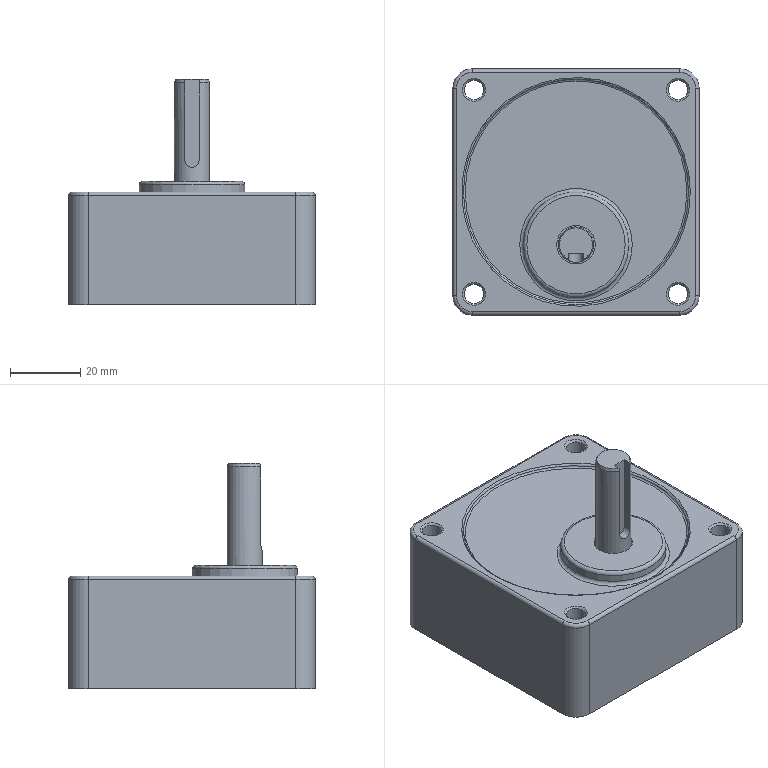Part | STEP file | S7KA3-18 | 1 solid | 46 faces | box 70 x 70 x 64 mm | volume 137824 mm3 | cylinder 18 | plane 15 | torus 8 | cone 5 | commonest cylinder face diameters 11 x5 2 x4 5.5 x4 4 x1 7 x1 10 x1
STEP:
#1=CARTESIAN_POINT('',(31.5,35.,5.));
#2=VERTEX_POINT('',#1);
#3=CARTESIAN_POINT('',(35.,35.,5.));
#4=DIRECTION('',(0.,0.,1.));
#5=DIRECTION('',(1.,0.,0.));
#6=AXIS2_PLACEMENT_3D('',#3,#4,#5);
#7=CIRCLE('',#6,3.5);
#8=EDGE_CURVE('',#2,#2,#7,.T.);
#9=ORIENTED_EDGE('',*,*,#8,.F.);
#10=CARTESIAN_POINT('',(31.5,35.,19.));
#11=VERTEX_POINT('',#10);
#12=CARTESIAN_POINT('',(31.5,35.,5.));
#13=DIRECTION('',(0.,0.,1.));
#14=VECTOR('',#13,3.5);
#15=LINE('',#12,#14);
#16=EDGE_CURVE('',#2,#11,#15,.T.);
#17=ORIENTED_EDGE('',*,*,#16,.T.);
#18=CARTESIAN_POINT('',(35.,35.,19.));
#19=DIRECTION('',(0.,0.,-1.));
#20=DIRECTION('',(1.,0.,0.));
#21=AXIS2_PLACEMENT_3D('',#18,#19,#20);
#22=CIRCLE('',#21,3.5);
#23=EDGE_CURVE('',#11,#11,#22,.T.);
#24=ORIENTED_EDGE('',*,*,#23,.F.);
#25=ORIENTED_EDGE('',*,*,#16,.F.);
#26=EDGE_LOOP('',(#9,#17,#24,#25));
#27=FACE_OUTER_BOUND('',#26,.T.);
#28=CARTESIAN_POINT('',(35.,35.,5.));
#29=DIRECTION('',(0.,0.,1.));
#30=DIRECTION('',(1.,0.,0.));
#31=AXIS2_PLACEMENT_3D('',#28,#29,#30);
#32=CYLINDRICAL_SURFACE('',#31,3.5);
#33=ADVANCED_FACE('',(#27),#32,.F.);
#34=ORIENTED_EDGE('',*,*,#23,.T.);
#35=EDGE_LOOP('',(#34));
#36=FACE_OUTER_BOUND('',#35,.T.);
#37=CARTESIAN_POINT('',(35.,35.,19.));
#38=DIRECTION('',(0.,0.,1.));
#39=DIRECTION('',(1.,0.,0.));
#40=AXIS2_PLACEMENT_3D('',#37,#38,#39);
#41=PLANE('',#40);
#42=ADVANCED_FACE('',(#36),#41,.F.);
#43=CARTESIAN_POINT('',(3.,35.,0.));
#44=VERTEX_POINT('',#43);
#45=CARTESIAN_POINT('',(35.,35.,0.));
#46=DIRECTION('',(0.,0.,1.));
#47=DIRECTION('',(1.,0.,0.));
#48=AXIS2_PLACEMENT_3D('',#45,#46,#47);
#49=CIRCLE('',#48,32.);
#50=EDGE_CURVE('',#44,#44,#49,.T.);
#51=ORIENTED_EDGE('',*,*,#50,.F.);
#52=CARTESIAN_POINT('',(3.,35.,5.));
#53=VERTEX_POINT('',#52);
#54=CARTESIAN_POINT('',(3.,35.,0.));
#55=DIRECTION('',(0.,0.,1.));
#56=VECTOR('',#55,32.);
#57=LINE('',#54,#56);
#58=EDGE_CURVE('',#44,#53,#57,.T.);
#59=ORIENTED_EDGE('',*,*,#58,.T.);
#60=CARTESIAN_POINT('',(35.,35.,5.));
#61=DIRECTION('',(0.,0.,-1.));
#62=DIRECTION('',(1.,0.,0.));
#63=AXIS2_PLACEMENT_3D('',#60,#61,#62);
#64=CIRCLE('',#63,32.);
#65=EDGE_CURVE('',#53,#53,#64,.T.);
#66=ORIENTED_EDGE('',*,*,#65,.F.);
#67=ORIENTED_EDGE('',*,*,#58,.F.);
#68=EDGE_LOOP('',(#51,#59,#66,#67));
#69=FACE_OUTER_BOUND('',#68,.T.);
#70=CARTESIAN_POINT('',(35.,35.,0.));
#71=DIRECTION('',(0.,0.,1.));
#72=DIRECTION('',(1.,0.,0.));
#73=AXIS2_PLACEMENT_3D('',#70,#71,#72);
#74=CYLINDRICAL_SURFACE('',#73,32.);
#75=ADVANCED_FACE('',(#69),#74,.F.);
#76=ORIENTED_EDGE('',*,*,#65,.T.);
#77=EDGE_LOOP('',(#76));
#78=FACE_OUTER_BOUND('',#77,.T.);
#79=ORIENTED_EDGE('',*,*,#8,.T.);
#80=EDGE_LOOP('',(#79));
#81=FACE_BOUND('',#80,.T.);
#82=CARTESIAN_POINT('',(35.,35.,5.));
#83=DIRECTION('',(0.,0.,1.));
#84=DIRECTION('',(1.,0.,0.));
#85=AXIS2_PLACEMENT_3D('',#82,#83,#84);
#86=PLANE('',#85);
#87=ADVANCED_FACE('',(#78,#81),#86,.F.);
#88=CARTESIAN_POINT('',(66.741,6.009,31.5));
#89=VERTEX_POINT('',#88);
#90=CARTESIAN_POINT('',(63.991,6.009,31.5));
#91=DIRECTION('',(0.,0.,-1.));
#92=DIRECTION('',(-1.,0.,0.));
#93=AXIS2_PLACEMENT_3D('',#90,#91,#92);
#94=CIRCLE('',#93,2.75);
#95=EDGE_CURVE('',#89,#89,#94,.T.);
#96=ORIENTED_EDGE('',*,*,#95,.T.);
#97=CARTESIAN_POINT('',(67.241,6.009,32.));
#98=VERTEX_POINT('',#97);
#99=CARTESIAN_POINT('',(66.991,6.009,31.75));
#100=DIRECTION('',(0.7071,0.,0.7071));
#101=VECTOR('',#100,3.);
#102=LINE('',#99,#101);
#103=EDGE_CURVE('',#89,#98,#102,.T.);
#104=ORIENTED_EDGE('',*,*,#103,.T.);
#105=CARTESIAN_POINT('',(63.991,6.009,32.));
#106=DIRECTION('',(0.,0.,1.));
#107=DIRECTION('',(-1.,0.,0.));
#108=AXIS2_PLACEMENT_3D('',#105,#106,#107);
#109=CIRCLE('',#108,3.25);
#110=EDGE_CURVE('',#98,#98,#109,.T.);
#111=ORIENTED_EDGE('',*,*,#110,.T.);
#112=ORIENTED_EDGE('',*,*,#103,.F.);
#113=EDGE_LOOP('',(#96,#104,#111,#112));
#114=FACE_OUTER_BOUND('',#113,.T.);
#115=CARTESIAN_POINT('',(63.991,6.009,31.75));
#116=DIRECTION('',(0.,0.,1.));
#117=DIRECTION('',(-1.,0.,0.));
#118=AXIS2_PLACEMENT_3D('',#115,#116,#117);
#119=CONICAL_SURFACE('',#118,3.,0.7854);
#120=ADVANCED_FACE('',(#114),#119,.F.);
#121=CARTESIAN_POINT('',(64.5,1.,32.));
#122=VERTEX_POINT('',#121);
#123=CARTESIAN_POINT('',(5.5,1.,32.));
#124=VERTEX_POINT('',#123);
#125=CARTESIAN_POINT('',(64.5,1.,32.));
#126=DIRECTION('',(-1.,0.,0.));
#127=VECTOR('',#126,59.);
#128=LINE('',#125,#127);
#129=EDGE_CURVE('',#122,#124,#128,.T.);
#130=ORIENTED_EDGE('',*,*,#129,.F.);
#131=CARTESIAN_POINT('',(69.,5.5,32.));
#132=VERTEX_POINT('',#131);
#133=CARTESIAN_POINT('',(64.5,5.5,32.));
#134=DIRECTION('',(0.,0.,-1.));
#135=DIRECTION('',(0.7071,-0.7071,0.));
#136=AXIS2_PLACEMENT_3D('',#133,#134,#135);
#137=CIRCLE('',#136,4.5);
#138=EDGE_CURVE('',#132,#122,#137,.T.);
#139=ORIENTED_EDGE('',*,*,#138,.F.);
#140=CARTESIAN_POINT('',(69.,64.5,32.));
#141=VERTEX_POINT('',#140);
#142=CARTESIAN_POINT('',(69.,64.5,32.));
#143=DIRECTION('',(0.,-1.,0.));
#144=VECTOR('',#143,59.);
#145=LINE('',#142,#144);
#146=EDGE_CURVE('',#141,#132,#145,.T.);
#147=ORIENTED_EDGE('',*,*,#146,.F.);
#148=CARTESIAN_POINT('',(64.5,69.,32.));
#149=VERTEX_POINT('',#148);
#150=CARTESIAN_POINT('',(64.5,64.5,32.));
#151=DIRECTION('',(0.,0.,-1.));
#152=DIRECTION('',(0.7071,0.7071,0.));
#153=AXIS2_PLACEMENT_3D('',#150,#151,#152);
#154=CIRCLE('',#153,4.5);
#155=EDGE_CURVE('',#149,#141,#154,.T.);
#156=ORIENTED_EDGE('',*,*,#155,.F.);
#157=CARTESIAN_POINT('',(5.5,69.,32.));
#158=VERTEX_POINT('',#157);
#159=CARTESIAN_POINT('',(5.5,69.,32.));
#160=DIRECTION('',(1.,0.,0.));
#161=VECTOR('',#160,59.);
#162=LINE('',#159,#161);
#163=EDGE_CURVE('',#158,#149,#162,.T.);
#164=ORIENTED_EDGE('',*,*,#163,.F.);
#165=CARTESIAN_POINT('',(1.,64.5,32.));
#166=VERTEX_POINT('',#165);
#167=CARTESIAN_POINT('',(5.5,64.5,32.));
#168=DIRECTION('',(0.,0.,-1.));
#169=DIRECTION('',(-0.7071,0.7071,0.));
#170=AXIS2_PLACEMENT_3D('',#167,#168,#169);
#171=CIRCLE('',#170,4.5);
#172=EDGE_CURVE('',#166,#158,#171,.T.);
#173=ORIENTED_EDGE('',*,*,#172,.F.);
#174=CARTESIAN_POINT('',(1.,5.5,32.));
#175=VERTEX_POINT('',#174);
#176=CARTESIAN_POINT('',(1.,5.5,32.));
#177=DIRECTION('',(0.,1.,0.));
#178=VECTOR('',#177,59.);
#179=LINE('',#176,#178);
#180=EDGE_CURVE('',#175,#166,#179,.T.);
#181=ORIENTED_EDGE('',*,*,#180,.F.);
#182=CARTESIAN_POINT('',(5.5,5.5,32.));
#183=DIRECTION('',(0.,0.,-1.));
#184=DIRECTION('',(-0.7071,-0.7071,0.));
#185=AXIS2_PLACEMENT_3D('',#182,#183,#184);
#186=CIRCLE('',#185,4.5);
#187=EDGE_CURVE('',#124,#175,#186,.T.);
#188=ORIENTED_EDGE('',*,*,#187,.F.);
#189=EDGE_LOOP('',(#130,#139,#147,#156,#164,#173,#181,#188));
#190=FACE_OUTER_BOUND('',#189,.T.);
#191=CARTESIAN_POINT('',(9.259,6.009,32.));
#192=VERTEX_POINT('',#191);
#193=CARTESIAN_POINT('',(6.009,6.009,32.));
#194=DIRECTION('',(0.,0.,1.));
#195=DIRECTION('',(-1.,0.,0.));
#196=AXIS2_PLACEMENT_3D('',#193,#194,#195);
#197=CIRCLE('',#196,3.25);
#198=EDGE_CURVE('',#192,#192,#197,.T.);
#199=ORIENTED_EDGE('',*,*,#198,.F.);
#200=EDGE_LOOP('',(#199));
#201=FACE_BOUND('',#200,.T.);
#202=CARTESIAN_POINT('',(67.241,63.991,32.));
#203=VERTEX_POINT('',#202);
#204=CARTESIAN_POINT('',(63.991,63.991,32.));
#205=DIRECTION('',(0.,0.,1.));
#206=DIRECTION('',(-1.,0.,0.));
#207=AXIS2_PLACEMENT_3D('',#204,#205,#206);
#208=CIRCLE('',#207,3.25);
#209=EDGE_CURVE('',#203,#203,#208,.T.);
#210=ORIENTED_EDGE('',*,*,#209,.F.);
#211=EDGE_LOOP('',(#210));
#212=FACE_BOUND('',#211,.T.);
#213=CARTESIAN_POINT('',(67.5,35.,32.));
#214=VERTEX_POINT('',#213);
#215=CARTESIAN_POINT('',(35.,35.,32.));
#216=DIRECTION('',(0.,0.,1.));
#217=DIRECTION('',(-1.,0.,0.));
#218=AXIS2_PLACEMENT_3D('',#215,#216,#217);
#219=CIRCLE('',#218,32.5);
#220=EDGE_CURVE('',#214,#214,#219,.T.);
#221=ORIENTED_EDGE('',*,*,#220,.F.);
#222=EDGE_LOOP('',(#221));
#223=FACE_BOUND('',#222,.T.);
#224=CARTESIAN_POINT('',(9.259,63.991,32.));
#225=VERTEX_POINT('',#224);
#226=CARTESIAN_POINT('',(6.009,63.991,32.));
#227=DIRECTION('',(0.,0.,1.));
#228=DIRECTION('',(-1.,0.,0.));
#229=AXIS2_PLACEMENT_3D('',#226,#227,#228);
#230=CIRCLE('',#229,3.25);
#231=EDGE_CURVE('',#225,#225,#230,.T.);
#232=ORIENTED_EDGE('',*,*,#231,.F.);
#233=EDGE_LOOP('',(#232));
#234=FACE_BOUND('',#233,.T.);
#235=ORIENTED_EDGE('',*,*,#110,.F.);
#236=EDGE_LOOP('',(#235));
#237=FACE_BOUND('',#236,.T.);
#238=CARTESIAN_POINT('',(35.,35.,32.));
#239=DIRECTION('',(0.,0.,1.));
#240=DIRECTION('',(1.,0.,0.));
#241=AXIS2_PLACEMENT_3D('',#238,#239,#240);
#242=PLANE('',#241);
#243=ADVANCED_FACE('',(#190,#201,#212,#223,#234,#237),#242,.T.);
#244=ORIENTED_EDGE('',*,*,#95,.F.);
#245=CARTESIAN_POINT('',(66.741,6.009,0.));
#246=VERTEX_POINT('',#245);
#247=CARTESIAN_POINT('',(66.741,6.009,32.));
#248=DIRECTION('',(0.,0.,-1.));
#249=VECTOR('',#248,2.75);
#250=LINE('',#247,#249);
#251=EDGE_CURVE('',#89,#246,#250,.T.);
#252=ORIENTED_EDGE('',*,*,#251,.T.);
#253=CARTESIAN_POINT('',(63.991,6.009,0.));
#254=DIRECTION('',(0.,0.,1.));
#255=DIRECTION('',(-1.,0.,0.));
#256=AXIS2_PLACEMENT_3D('',#253,#254,#255);
#257=CIRCLE('',#256,2.75);
#258=EDGE_CURVE('',#246,#246,#257,.T.);
#259=ORIENTED_EDGE('',*,*,#258,.F.);
#260=ORIENTED_EDGE('',*,*,#251,.F.);
#261=EDGE_LOOP('',(#244,#252,#259,#260));
#262=FACE_OUTER_BOUND('',#261,.T.);
#263=CARTESIAN_POINT('',(63.991,6.009,32.));
#264=DIRECTION('',(0.,0.,-1.));
#265=DIRECTION('',(-1.,0.,0.));
#266=AXIS2_PLACEMENT_3D('',#263,#264,#265);
#267=CYLINDRICAL_SURFACE('',#266,2.75);
#268=ADVANCED_FACE('',(#262),#267,.F.);
#269=CARTESIAN_POINT('',(8.759,6.009,31.5));
#270=VERTEX_POINT('',#269);
#271=CARTESIAN_POINT('',(6.009,6.009,31.5));
#272=DIRECTION('',(0.,0.,-1.));
#273=DIRECTION('',(-1.,0.,0.));
#274=AXIS2_PLACEMENT_3D('',#271,#272,#273);
#275=CIRCLE('',#274,2.75);
#276=EDGE_CURVE('',#270,#270,#275,.T.);
#277=ORIENTED_EDGE('',*,*,#276,.T.);
#278=CARTESIAN_POINT('',(9.009,6.009,31.75));
#279=DIRECTION('',(0.7071,0.,0.7071));
#280=VECTOR('',#279,3.);
#281=LINE('',#278,#280);
#282=EDGE_CURVE('',#270,#192,#281,.T.);
#283=ORIENTED_EDGE('',*,*,#282,.T.);
#284=ORIENTED_EDGE('',*,*,#198,.T.);
#285=ORIENTED_EDGE('',*,*,#282,.F.);
#286=EDGE_LOOP('',(#277,#283,#284,#285));
#287=FACE_OUTER_BOUND('',#286,.T.);
#288=CARTESIAN_POINT('',(6.009,6.009,31.75));
#289=DIRECTION('',(0.,0.,1.));
#290=DIRECTION('',(-1.,0.,0.));
#291=AXIS2_PLACEMENT_3D('',#288,#289,#290);
#292=CONICAL_SURFACE('',#291,3.,0.7854);
#293=ADVANCED_FACE('',(#287),#292,.F.);
#294=ORIENTED_EDGE('',*,*,#276,.F.);
#295=CARTESIAN_POINT('',(8.759,6.009,0.));
#296=VERTEX_POINT('',#295);
#297=CARTESIAN_POINT('',(8.759,6.009,32.));
#298=DIRECTION('',(0.,0.,-1.));
#299=VECTOR('',#298,2.75);
#300=LINE('',#297,#299);
#301=EDGE_CURVE('',#270,#296,#300,.T.);
#302=ORIENTED_EDGE('',*,*,#301,.T.);
#303=CARTESIAN_POINT('',(6.009,6.009,0.));
#304=DIRECTION('',(0.,0.,1.));
#305=DIRECTION('',(-1.,0.,0.));
#306=AXIS2_PLACEMENT_3D('',#303,#304,#305);
#307=CIRCLE('',#306,2.75);
#308=EDGE_CURVE('',#296,#296,#307,.T.);
#309=ORIENTED_EDGE('',*,*,#308,.F.);
#310=ORIENTED_EDGE('',*,*,#301,.F.);
#311=EDGE_LOOP('',(#294,#302,#309,#310));
#312=FACE_OUTER_BOUND('',#311,.T.);
#313=CARTESIAN_POINT('',(6.009,6.009,32.));
#314=DIRECTION('',(0.,0.,-1.));
#315=DIRECTION('',(-1.,0.,0.));
#316=AXIS2_PLACEMENT_3D('',#313,#314,#315);
#317=CYLINDRICAL_SURFACE('',#316,2.75);
#318=ADVANCED_FACE('',(#312),#317,.F.);
#319=CARTESIAN_POINT('',(8.759,63.991,31.5));
#320=VERTEX_POINT('',#319);
#321=CARTESIAN_POINT('',(6.009,63.991,31.5));
#322=DIRECTION('',(0.,0.,-1.));
#323=DIRECTION('',(-1.,0.,0.));
#324=AXIS2_PLACEMENT_3D('',#321,#322,#323);
#325=CIRCLE('',#324,2.75);
#326=EDGE_CURVE('',#320,#320,#325,.T.);
#327=ORIENTED_EDGE('',*,*,#326,.T.);
#328=CARTESIAN_POINT('',(9.009,63.991,31.75));
#329=DIRECTION('',(0.7071,0.,0.7071));
#330=VECTOR('',#329,3.);
#331=LINE('',#328,#330);
#332=EDGE_CURVE('',#320,#225,#331,.T.);
#333=ORIENTED_EDGE('',*,*,#332,.T.);
#334=ORIENTED_EDGE('',*,*,#231,.T.);
#335=ORIENTED_EDGE('',*,*,#332,.F.);
#336=EDGE_LOOP('',(#327,#333,#334,#335));
#337=FACE_OUTER_BOUND('',#336,.T.);
#338=CARTESIAN_POINT('',(6.009,63.991,31.75));
#339=DIRECTION('',(0.,0.,1.));
#340=DIRECTION('',(-1.,0.,0.));
#341=AXIS2_PLACEMENT_3D('',#338,#339,#340);
#342=CONICAL_SURFACE('',#341,3.,0.7854);
#343=ADVANCED_FACE('',(#337),#342,.F.);
#344=ORIENTED_EDGE('',*,*,#326,.F.);
#345=CARTESIAN_POINT('',(8.759,63.991,0.));
#346=VERTEX_POINT('',#345);
#347=CARTESIAN_POINT('',(8.759,63.991,32.));
#348=DIRECTION('',(0.,0.,-1.));
#349=VECTOR('',#348,2.75);
#350=LINE('',#347,#349);
#351=EDGE_CURVE('',#320,#346,#350,.T.);
#352=ORIENTED_EDGE('',*,*,#351,.T.);
#353=CARTESIAN_POINT('',(6.009,63.991,0.));
#354=DIRECTION('',(0.,0.,1.));
#355=DIRECTION('',(-1.,0.,0.));
#356=AXIS2_PLACEMENT_3D('',#353,#354,#355);
#357=CIRCLE('',#356,2.75);
#358=EDGE_CURVE('',#346,#346,#357,.T.);
#359=ORIENTED_EDGE('',*,*,#358,.F.);
#360=ORIENTED_EDGE('',*,*,#351,.F.);
#361=EDGE_LOOP('',(#344,#352,#359,#360));
#362=FACE_OUTER_BOUND('',#361,.T.);
#363=CARTESIAN_POINT('',(6.009,63.991,32.));
#364=DIRECTION('',(0.,0.,-1.));
#365=DIRECTION('',(-1.,0.,0.));
#366=AXIS2_PLACEMENT_3D('',#363,#364,#365);
#367=CYLINDRICAL_SURFACE('',#366,2.75);
#368=ADVANCED_FACE('',(#362),#367,.F.);
#369=CARTESIAN_POINT('',(66.741,63.991,31.5));
#370=VERTEX_POINT('',#369);
#371=CARTESIAN_POINT('',(63.991,63.991,31.5));
#372=DIRECTION('',(0.,0.,-1.));
#373=DIRECTION('',(-1.,0.,0.));
#374=AXIS2_PLACEMENT_3D('',#371,#372,#373);
#375=CIRCLE('',#374,2.75);
#376=EDGE_CURVE('',#370,#370,#375,.T.);
#377=ORIENTED_EDGE('',*,*,#376,.T.);
#378=CARTESIAN_POINT('',(66.991,63.991,31.75));
#379=DIRECTION('',(0.7071,0.,0.7071));
#380=VECTOR('',#379,3.);
#381=LINE('',#378,#380);
#382=EDGE_CURVE('',#370,#203,#381,.T.);
#383=ORIENTED_EDGE('',*,*,#382,.T.);
#384=ORIENTED_EDGE('',*,*,#209,.T.);
#385=ORIENTED_EDGE('',*,*,#382,.F.);
#386=EDGE_LOOP('',(#377,#383,#384,#385));
#387=FACE_OUTER_BOUND('',#386,.T.);
#388=CARTESIAN_POINT('',(63.991,63.991,31.75));
#389=DIRECTION('',(0.,0.,1.));
#390=DIRECTION('',(-1.,0.,0.));
#391=AXIS2_PLACEMENT_3D('',#388,#389,#390);
#392=CONICAL_SURFACE('',#391,3.,0.7854);
#393=ADVANCED_FACE('',(#387),#392,.F.);
#394=ORIENTED_EDGE('',*,*,#376,.F.);
#395=CARTESIAN_POINT('',(66.741,63.991,0.));
#396=VERTEX_POINT('',#395);
#397=CARTESIAN_POINT('',(66.741,63.991,32.));
#398=DIRECTION('',(0.,0.,-1.));
#399=VECTOR('',#398,2.75);
#400=LINE('',#397,#399);
#401=EDGE_CURVE('',#370,#396,#400,.T.);
#402=ORIENTED_EDGE('',*,*,#401,.T.);
#403=CARTESIAN_POINT('',(63.991,63.991,0.));
#404=DIRECTION('',(0.,0.,1.));
#405=DIRECTION('',(-1.,0.,0.));
#406=AXIS2_PLACEMENT_3D('',#403,#404,#405);
#407=CIRCLE('',#406,2.75);
#408=EDGE_CURVE('',#396,#396,#407,.T.);
#409=ORIENTED_EDGE('',*,*,#408,.F.);
#410=ORIENTED_EDGE('',*,*,#401,.F.);
#411=EDGE_LOOP('',(#394,#402,#409,#410));
#412=FACE_OUTER_BOUND('',#411,.T.);
#413=CARTESIAN_POINT('',(63.991,63.991,32.));
#414=DIRECTION('',(0.,0.,-1.));
#415=DIRECTION('',(-1.,0.,0.));
#416=AXIS2_PLACEMENT_3D('',#413,#414,#415);
#417=CYLINDRICAL_SURFACE('',#416,2.75);
#418=ADVANCED_FACE('',(#412),#417,.F.);
#419=CARTESIAN_POINT('',(33.,15.417,41.));
#420=VERTEX_POINT('',#419);
#421=CARTESIAN_POINT('',(33.,15.417,63.));
#422=VERTEX_POINT('',#421);
#423=CARTESIAN_POINT('',(33.,15.417,41.));
#424=DIRECTION('',(0.,0.,1.));
#425=VECTOR('',#424,22.);
#426=LINE('',#423,#425);
#427=EDGE_CURVE('',#420,#422,#426,.T.);
#428=ORIENTED_EDGE('',*,*,#427,.F.);
#429=CARTESIAN_POINT('',(33.,17.5,41.));
#430=VERTEX_POINT('',#429);
#431=CARTESIAN_POINT('',(33.,15.417,41.));
#432=DIRECTION('',(0.,1.,0.));
#433=VECTOR('',#432,2.083);
#434=LINE('',#431,#433);
#435=EDGE_CURVE('',#420,#430,#434,.T.);
#436=ORIENTED_EDGE('',*,*,#435,.T.);
#437=CARTESIAN_POINT('',(33.,17.5,64.));
#438=VERTEX_POINT('',#437);
#439=CARTESIAN_POINT('',(33.,17.5,64.));
#440=DIRECTION('',(0.,0.,-1.));
#441=VECTOR('',#440,23.);
#442=LINE('',#439,#441);
#443=EDGE_CURVE('',#438,#430,#442,.T.);
#444=ORIENTED_EDGE('',*,*,#443,.F.);
#445=CARTESIAN_POINT('',(33.,15.711,64.));
#446=VERTEX_POINT('',#445);
#447=CARTESIAN_POINT('',(33.,15.711,64.));
#448=DIRECTION('',(0.,1.,0.));
#449=VECTOR('',#448,1.789);
#450=LINE('',#447,#449);
#451=EDGE_CURVE('',#446,#438,#450,.T.);
#452=ORIENTED_EDGE('',*,*,#451,.F.);
#453=CARTESIAN_POINT('',(33.,15.417,63.));
#454=CARTESIAN_POINT('',(33.,15.568,63.517));
#455=CARTESIAN_POINT('',(33.,15.711,64.));
#456=(BOUNDED_CURVE()B_SPLINE_CURVE(2,(#453,#454,#455),.UNSPECIFIED.,.F.,.F.)B_SPLINE_CURVE_WITH_KNOTS((3,3),(2.267,2.427),.UNSPECIFIED.)CURVE()GEOMETRIC_REPRESENTATION_ITEM()RATIONAL_B_SPLINE_CURVE((1.026,1.021,1.014))REPRESENTATION_ITEM(''));
#457=EDGE_CURVE('',#422,#446,#456,.T.);
#458=ORIENTED_EDGE('',*,*,#457,.F.);
#459=EDGE_LOOP('',(#428,#436,#444,#452,#458));
#460=FACE_OUTER_BOUND('',#459,.T.);
#461=CARTESIAN_POINT('',(33.,15.,64.));
#462=DIRECTION('',(-1.,0.,0.));
#463=DIRECTION('',(0.,0.,1.));
#464=AXIS2_PLACEMENT_3D('',#461,#462,#463);
#465=PLANE('',#464);
#466=ADVANCED_FACE('',(#460),#465,.F.);
#467=CARTESIAN_POINT('',(37.,15.417,41.));
#468=VERTEX_POINT('',#467);
#469=CARTESIAN_POINT('',(33.,15.417,41.));
#470=CARTESIAN_POINT('',(33.,15.417,40.746));
#471=CARTESIAN_POINT('',(33.051,15.394,40.477));
#472=CARTESIAN_POINT('',(33.256,15.313,39.985));
#473=CARTESIAN_POINT('',(33.41,15.256,39.762));
#474=CARTESIAN_POINT('',(33.762,15.152,39.41));
#475=CARTESIAN_POINT('',(33.985,15.098,39.256));
#476=CARTESIAN_POINT('',(34.477,15.021,39.051));
#477=CARTESIAN_POINT('',(34.746,15.,39.));
#478=CARTESIAN_POINT('',(35.254,15.,39.));
#479=CARTESIAN_POINT('',(35.523,15.021,39.051));
#480=CARTESIAN_POINT('',(36.015,15.098,39.256));
#481=CARTESIAN_POINT('',(36.238,15.152,39.41));
#482=CARTESIAN_POINT('',(36.59,15.256,39.762));
#483=CARTESIAN_POINT('',(36.744,15.313,39.985));
#484=CARTESIAN_POINT('',(36.949,15.394,40.477));
#485=CARTESIAN_POINT('',(37.,15.417,40.746));
#486=CARTESIAN_POINT('',(37.,15.417,41.));
#487=B_SPLINE_CURVE_WITH_KNOTS('',3,(#469,#470,#471,#472,#473,#474,#475,#476,#477,#478,#479,#480,#481,#482,#483,#484,#485,#486),.UNSPECIFIED.,.F.,.F.,(4,2,2,2,2,2,2,2,4),(-1.22,-1.144,-1.068,-0.9915,-0.9153,-0.839,-0.7628,-0.6865,-0.6102),.UNSPECIFIED.);
#488=EDGE_CURVE('',#468,#420,#487,.F.);
#489=ORIENTED_EDGE('',*,*,#488,.F.);
#490=CARTESIAN_POINT('',(37.,17.5,41.));
#491=VERTEX_POINT('',#490);
#492=CARTESIAN_POINT('',(37.,15.417,41.));
#493=DIRECTION('',(0.,1.,0.));
#494=VECTOR('',#493,2.083);
#495=LINE('',#492,#494);
#496=EDGE_CURVE('',#468,#491,#495,.T.);
#497=ORIENTED_EDGE('',*,*,#496,.T.);
#498=CARTESIAN_POINT('',(35.,17.5,41.));
#499=DIRECTION('',(0.,-1.,0.));
#500=DIRECTION('',(-1.,0.,0.));
#501=AXIS2_PLACEMENT_3D('',#498,#499,#500);
#502=CIRCLE('',#501,2.);
#503=EDGE_CURVE('',#430,#491,#502,.T.);
#504=ORIENTED_EDGE('',*,*,#503,.F.);
#505=ORIENTED_EDGE('',*,*,#435,.F.);
#506=EDGE_LOOP('',(#489,#497,#504,#505));
#507=FACE_OUTER_BOUND('',#506,.T.);
#508=CARTESIAN_POINT('',(35.,15.,41.));
#509=DIRECTION('',(0.,1.,0.));
#510=DIRECTION('',(-1.,0.,0.));
#511=AXIS2_PLACEMENT_3D('',#508,#509,#510);
#512=CYLINDRICAL_SURFACE('',#511,2.);
#513=ADVANCED_FACE('',(#507),#512,.F.);
#514=CARTESIAN_POINT('',(37.,15.417,63.));
#515=VERTEX_POINT('',#514);
#516=CARTESIAN_POINT('',(37.,15.417,63.));
#517=DIRECTION('',(0.,0.,-1.));
#518=VECTOR('',#517,22.);
#519=LINE('',#516,#518);
#520=EDGE_CURVE('',#515,#468,#519,.T.);
#521=ORIENTED_EDGE('',*,*,#520,.F.);
#522=CARTESIAN_POINT('',(37.,15.711,64.));
#523=VERTEX_POINT('',#522);
#524=CARTESIAN_POINT('',(37.,15.711,64.));
#525=CARTESIAN_POINT('',(37.,15.568,63.517));
#526=CARTESIAN_POINT('',(37.,15.417,63.));
#527=(BOUNDED_CURVE()B_SPLINE_CURVE(2,(#524,#525,#526),.UNSPECIFIED.,.F.,.F.)B_SPLINE_CURVE_WITH_KNOTS((3,3),(0.1692,0.3292),.UNSPECIFIED.)CURVE()GEOMETRIC_REPRESENTATION_ITEM()RATIONAL_B_SPLINE_CURVE((1.014,1.021,1.026))REPRESENTATION_ITEM(''));
#528=EDGE_CURVE('',#523,#515,#527,.T.);
#529=ORIENTED_EDGE('',*,*,#528,.F.);
#530=CARTESIAN_POINT('',(37.,17.5,64.));
#531=VERTEX_POINT('',#530);
#532=CARTESIAN_POINT('',(37.,17.5,64.));
#533=DIRECTION('',(0.,-1.,0.));
#534=VECTOR('',#533,1.789);
#535=LINE('',#532,#534);
#536=EDGE_CURVE('',#531,#523,#535,.T.);
#537=ORIENTED_EDGE('',*,*,#536,.F.);
#538=CARTESIAN_POINT('',(37.,17.5,41.));
#539=DIRECTION('',(0.,0.,1.));
#540=VECTOR('',#539,23.);
#541=LINE('',#538,#540);
#542=EDGE_CURVE('',#491,#531,#541,.T.);
#543=ORIENTED_EDGE('',*,*,#542,.F.);
#544=ORIENTED_EDGE('',*,*,#496,.F.);
#545=EDGE_LOOP('',(#521,#529,#537,#543,#544));
#546=FACE_OUTER_BOUND('',#545,.T.);
#547=CARTESIAN_POINT('',(37.,15.,41.));
#548=DIRECTION('',(1.,0.,0.));
#549=DIRECTION('',(0.,0.,-1.));
#550=AXIS2_PLACEMENT_3D('',#547,#548,#549);
#551=PLANE('',#550);
#552=ADVANCED_FACE('',(#546),#551,.F.);
#553=ORIENTED_EDGE('',*,*,#443,.T.);
#554=ORIENTED_EDGE('',*,*,#503,.T.);
#555=ORIENTED_EDGE('',*,*,#542,.T.);
#556=CARTESIAN_POINT('',(33.,17.5,64.));
#557=DIRECTION('',(1.,0.,0.));
#558=VECTOR('',#557,4.);
#559=LINE('',#556,#558);
#560=EDGE_CURVE('',#438,#531,#559,.T.);
#561=ORIENTED_EDGE('',*,*,#560,.F.);
#562=EDGE_LOOP('',(#553,#554,#555,#561));
#563=FACE_OUTER_BOUND('',#562,.T.);
#564=CARTESIAN_POINT('',(35.,17.5,51.905));
#565=DIRECTION('',(0.,1.,0.));
#566=DIRECTION('',(0.,0.,1.));
#567=AXIS2_PLACEMENT_3D('',#564,#565,#566);
#568=PLANE('',#567);
#569=ADVANCED_FACE('',(#563),#568,.F.);
#570=CARTESIAN_POINT('',(40.,20.,63.));
#571=VERTEX_POINT('',#570);
#572=CARTESIAN_POINT('',(35.,20.,63.));
#573=DIRECTION('',(0.,0.,-1.));
#574=DIRECTION('',(-1.,0.,0.));
#575=AXIS2_PLACEMENT_3D('',#572,#573,#574);
#576=CIRCLE('',#575,5.);
#577=EDGE_CURVE('',#422,#571,#576,.T.);
#578=ORIENTED_EDGE('',*,*,#577,.T.);
#579=CARTESIAN_POINT('',(40.,20.,31.));
#580=VERTEX_POINT('',#579);
#581=CARTESIAN_POINT('',(40.,20.,31.));
#582=DIRECTION('',(0.,0.,-1.));
#583=VECTOR('',#582,5.);
#584=LINE('',#581,#583);
#585=EDGE_CURVE('',#571,#580,#584,.T.);
#586=ORIENTED_EDGE('',*,*,#585,.T.);
#587=CARTESIAN_POINT('',(35.,20.,31.));
#588=DIRECTION('',(0.,0.,-1.));
#589=DIRECTION('',(-1.,0.,0.));
#590=AXIS2_PLACEMENT_3D('',#587,#588,#589);
#591=CIRCLE('',#590,5.);
#592=EDGE_CURVE('',#580,#580,#591,.T.);
#593=ORIENTED_EDGE('',*,*,#592,.F.);
#594=ORIENTED_EDGE('',*,*,#585,.F.);
#595=CARTESIAN_POINT('',(35.,20.,63.));
#596=DIRECTION('',(0.,0.,-1.));
#597=DIRECTION('',(-1.,0.,0.));
#598=AXIS2_PLACEMENT_3D('',#595,#596,#597);
#599=CIRCLE('',#598,5.);
#600=EDGE_CURVE('',#571,#515,#599,.T.);
#601=ORIENTED_EDGE('',*,*,#600,.T.);
#602=ORIENTED_EDGE('',*,*,#520,.T.);
#603=ORIENTED_EDGE('',*,*,#488,.T.);
#604=ORIENTED_EDGE('',*,*,#427,.T.);
#605=EDGE_LOOP('',(#578,#586,#593,#594,#601,#602,#603,#604));
#606=FACE_OUTER_BOUND('',#605,.T.);
#607=CARTESIAN_POINT('',(35.,20.,31.));
#608=DIRECTION('',(0.,0.,1.));
#609=DIRECTION('',(-1.,0.,0.));
#610=AXIS2_PLACEMENT_3D('',#607,#608,#609);
#611=CYLINDRICAL_SURFACE('',#610,5.);
#612=ADVANCED_FACE('',(#606),#611,.T.);
#613=ORIENTED_EDGE('',*,*,#451,.T.);
#614=ORIENTED_EDGE('',*,*,#560,.T.);
#615=ORIENTED_EDGE('',*,*,#536,.T.);
#616=CARTESIAN_POINT('',(35.,20.,64.));
#617=DIRECTION('',(0.,0.,-1.));
#618=DIRECTION('',(-1.,0.,0.));
#619=AXIS2_PLACEMENT_3D('',#616,#617,#618);
#620=CIRCLE('',#619,4.732);
#621=EDGE_CURVE('',#446,#523,#620,.T.);
#622=ORIENTED_EDGE('',*,*,#621,.F.);
#623=EDGE_LOOP('',(#613,#614,#615,#622));
#624=FACE_OUTER_BOUND('',#623,.T.);
#625=CARTESIAN_POINT('',(35.,20.,64.));
#626=DIRECTION('',(0.,0.,-1.));
#627=DIRECTION('',(-1.,0.,0.));
#628=AXIS2_PLACEMENT_3D('',#625,#626,#627);
#629=PLANE('',#628);
#630=ADVANCED_FACE('',(#624),#629,.F.);
#631=ORIENTED_EDGE('',*,*,#457,.T.);
#632=ORIENTED_EDGE('',*,*,#621,.T.);
#633=ORIENTED_EDGE('',*,*,#528,.T.);
#634=ORIENTED_EDGE('',*,*,#600,.F.);
#635=ORIENTED_EDGE('',*,*,#577,.F.);
#636=EDGE_LOOP('',(#631,#632,#633,#634,#635));
#637=FACE_OUTER_BOUND('',#636,.T.);
#638=CARTESIAN_POINT('',(35.,20.,63.));
#639=DIRECTION('',(0.,0.,-1.));
#640=DIRECTION('',(0.,1.,0.));
#641=AXIS2_PLACEMENT_3D('',#638,#639,#640);
#642=CONICAL_SURFACE('',#641,5.,0.2618);
#643=ADVANCED_FACE('',(#637),#642,.T.);
#644=CARTESIAN_POINT('',(51.,20.,31.));
#645=VERTEX_POINT('',#644);
#646=CARTESIAN_POINT('',(35.,20.,31.));
#647=DIRECTION('',(0.,0.,1.));
#648=DIRECTION('',(-1.,0.,0.));
#649=AXIS2_PLACEMENT_3D('',#646,#647,#648);
#650=CIRCLE('',#649,16.);
#651=EDGE_CURVE('',#645,#645,#650,.T.);
#652=ORIENTED_EDGE('',*,*,#651,.T.);
#653=CARTESIAN_POINT('',(50.,20.,32.));
#654=VERTEX_POINT('',#653);
#655=CARTESIAN_POINT('',(51.,20.,32.));
#656=DIRECTION('',(0.,1.,0.));
#657=DIRECTION('',(1.,0.,0.));
#658=AXIS2_PLACEMENT_3D('',#655,#656,#657);
#659=CIRCLE('',#658,1.);
#660=EDGE_CURVE('',#645,#654,#659,.T.);
#661=ORIENTED_EDGE('',*,*,#660,.T.);
#662=CARTESIAN_POINT('',(35.,20.,32.));
#663=DIRECTION('',(0.,0.,-1.));
#664=DIRECTION('',(-1.,0.,0.));
#665=AXIS2_PLACEMENT_3D('',#662,#663,#664);
#666=CIRCLE('',#665,15.);
#667=EDGE_CURVE('',#654,#654,#666,.T.);
#668=ORIENTED_EDGE('',*,*,#667,.T.);
#669=ORIENTED_EDGE('',*,*,#660,.F.);
#670=EDGE_LOOP('',(#652,#661,#668,#669));
#671=FACE_OUTER_BOUND('',#670,.T.);
#672=CARTESIAN_POINT('',(35.,20.,32.));
#673=DIRECTION('',(0.,0.,-1.));
#674=DIRECTION('',(-1.,0.,0.));
#675=AXIS2_PLACEMENT_3D('',#672,#673,#674);
#676=TOROIDAL_SURFACE('',#675,16.,1.);
#677=ADVANCED_FACE('',(#671),#676,.F.);
#678=CARTESIAN_POINT('',(50.,20.,34.));
#679=VERTEX_POINT('',#678);
#680=CARTESIAN_POINT('',(35.,20.,34.));
#681=DIRECTION('',(0.,0.,1.));
#682=DIRECTION('',(-1.,0.,0.));
#683=AXIS2_PLACEMENT_3D('',#680,#681,#682);
#684=CIRCLE('',#683,15.);
#685=EDGE_CURVE('',#679,#679,#684,.T.);
#686=ORIENTED_EDGE('',*,*,#685,.F.);
#687=CARTESIAN_POINT('',(50.,20.,31.));
#688=DIRECTION('',(0.,0.,-1.));
#689=VECTOR('',#688,15.);
#690=LINE('',#687,#689);
#691=EDGE_CURVE('',#679,#654,#690,.T.);
#692=ORIENTED_EDGE('',*,*,#691,.T.);
#693=ORIENTED_EDGE('',*,*,#667,.F.);
#694=ORIENTED_EDGE('',*,*,#691,.F.);
#695=EDGE_LOOP('',(#686,#692,#693,#694));
#696=FACE_OUTER_BOUND('',#695,.T.);
#697=CARTESIAN_POINT('',(35.,20.,31.));
#698=DIRECTION('',(0.,0.,1.));
#699=DIRECTION('',(-1.,0.,0.));
#700=AXIS2_PLACEMENT_3D('',#697,#698,#699);
#701=CYLINDRICAL_SURFACE('',#700,15.);
#702=ADVANCED_FACE('',(#696),#701,.T.);
#703=CARTESIAN_POINT('',(66.5,35.,31.));
#704=VERTEX_POINT('',#703);
#705=CARTESIAN_POINT('',(3.5,35.,31.));
#706=VERTEX_POINT('',#705);
#707=CARTESIAN_POINT('',(35.,35.,31.));
#708=DIRECTION('',(0.,0.,-1.));
#709=DIRECTION('',(-1.,0.,0.));
#710=AXIS2_PLACEMENT_3D('',#707,#708,#709);
#711=CIRCLE('',#710,31.5);
#712=EDGE_CURVE('',#704,#706,#711,.T.);
#713=ORIENTED_EDGE('',*,*,#712,.F.);
#714=CARTESIAN_POINT('',(35.,35.,31.));
#715=DIRECTION('',(0.,0.,-1.));
#716=DIRECTION('',(-1.,0.,0.));
#717=AXIS2_PLACEMENT_3D('',#714,#715,#716);
#718=CIRCLE('',#717,31.5);
#719=EDGE_CURVE('',#706,#704,#718,.T.);
#720=ORIENTED_EDGE('',*,*,#719,.F.);
#721=EDGE_LOOP('',(#713,#720));
#722=FACE_OUTER_BOUND('',#721,.T.);
#723=ORIENTED_EDGE('',*,*,#651,.F.);
#724=EDGE_LOOP('',(#723));
#725=FACE_BOUND('',#724,.T.);
#726=CARTESIAN_POINT('',(35.,35.,31.));
#727=DIRECTION('',(0.,0.,-1.));
#728=DIRECTION('',(-1.,0.,0.));
#729=AXIS2_PLACEMENT_3D('',#726,#727,#728);
#730=PLANE('',#729);
#731=ADVANCED_FACE('',(#722,#725),#730,.F.);
#732=ORIENTED_EDGE('',*,*,#685,.T.);
#733=CARTESIAN_POINT('',(49.,20.,35.));
#734=VERTEX_POINT('',#733);
#735=CARTESIAN_POINT('',(49.,20.,34.));
#736=DIRECTION('',(0.,-1.,0.));
#737=DIRECTION('',(1.,0.,0.));
#738=AXIS2_PLACEMENT_3D('',#735,#736,#737);
#739=CIRCLE('',#738,1.);
#740=EDGE_CURVE('',#679,#734,#739,.T.);
#741=ORIENTED_EDGE('',*,*,#740,.T.);
#742=CARTESIAN_POINT('',(35.,20.,35.));
#743=DIRECTION('',(0.,0.,-1.));
#744=DIRECTION('',(-1.,0.,0.));
#745=AXIS2_PLACEMENT_3D('',#742,#743,#744);
#746=CIRCLE('',#745,14.);
#747=EDGE_CURVE('',#734,#734,#746,.T.);
#748=ORIENTED_EDGE('',*,*,#747,.T.);
#749=ORIENTED_EDGE('',*,*,#740,.F.);
#750=EDGE_LOOP('',(#732,#741,#748,#749));
#751=FACE_OUTER_BOUND('',#750,.T.);
#752=CARTESIAN_POINT('',(35.,20.,34.));
#753=DIRECTION('',(0.,0.,-1.));
#754=DIRECTION('',(-1.,0.,0.));
#755=AXIS2_PLACEMENT_3D('',#752,#753,#754);
#756=TOROIDAL_SURFACE('',#755,14.,1.);
#757=ADVANCED_FACE('',(#751),#756,.T.);
#758=ORIENTED_EDGE('',*,*,#747,.F.);
#759=EDGE_LOOP('',(#758));
#760=FACE_OUTER_BOUND('',#759,.T.);
#761=CARTESIAN_POINT('',(40.5,20.,35.));
#762=VERTEX_POINT('',#761);
#763=CARTESIAN_POINT('',(35.,20.,35.));
#764=DIRECTION('',(0.,0.,-1.));
#765=DIRECTION('',(-1.,0.,0.));
#766=AXIS2_PLACEMENT_3D('',#763,#764,#765);
#767=CIRCLE('',#766,5.5);
#768=EDGE_CURVE('',#762,#762,#767,.T.);
#769=ORIENTED_EDGE('',*,*,#768,.T.);
#770=EDGE_LOOP('',(#769));
#771=FACE_BOUND('',#770,.T.);
#772=CARTESIAN_POINT('',(35.,20.,35.));
#773=DIRECTION('',(0.,0.,-1.));
#774=DIRECTION('',(-1.,0.,0.));
#775=AXIS2_PLACEMENT_3D('',#772,#773,#774);
#776=PLANE('',#775);
#777=ADVANCED_FACE('',(#760,#771),#776,.F.);
#778=CARTESIAN_POINT('',(40.5,20.,31.));
#779=VERTEX_POINT('',#778);
#780=CARTESIAN_POINT('',(35.,20.,31.));
#781=DIRECTION('',(0.,0.,1.));
#782=DIRECTION('',(-1.,0.,0.));
#783=AXIS2_PLACEMENT_3D('',#780,#781,#782);
#784=CIRCLE('',#783,5.5);
#785=EDGE_CURVE('',#779,#779,#784,.T.);
#786=ORIENTED_EDGE('',*,*,#785,.F.);
#787=CARTESIAN_POINT('',(40.5,20.,31.));
#788=DIRECTION('',(0.,0.,1.));
#789=VECTOR('',#788,5.5);
#790=LINE('',#787,#789);
#791=EDGE_CURVE('',#779,#762,#790,.T.);
#792=ORIENTED_EDGE('',*,*,#791,.T.);
#793=ORIENTED_EDGE('',*,*,#768,.F.);
#794=ORIENTED_EDGE('',*,*,#791,.F.);
#795=EDGE_LOOP('',(#786,#792,#793,#794));
#796=FACE_OUTER_BOUND('',#795,.T.);
#797=CARTESIAN_POINT('',(35.,20.,31.));
#798=DIRECTION('',(0.,0.,1.));
#799=DIRECTION('',(-1.,0.,0.));
#800=AXIS2_PLACEMENT_3D('',#797,#798,#799);
#801=CYLINDRICAL_SURFACE('',#800,5.5);
#802=ADVANCED_FACE('',(#796),#801,.F.);
#803=ORIENTED_EDGE('',*,*,#712,.T.);
#804=CARTESIAN_POINT('',(3.,35.,31.5));
#805=VERTEX_POINT('',#804);
#806=CARTESIAN_POINT('',(3.5,35.,31.5));
#807=DIRECTION('',(0.,1.,0.));
#808=DIRECTION('',(-1.,0.,0.));
#809=AXIS2_PLACEMENT_3D('',#806,#807,#808);
#810=CIRCLE('',#809,0.5);
#811=EDGE_CURVE('',#706,#805,#810,.T.);
#812=ORIENTED_EDGE('',*,*,#811,.T.);
#813=CARTESIAN_POINT('',(67.,35.,31.5));
#814=VERTEX_POINT('',#813);
#815=CARTESIAN_POINT('',(35.,35.,31.5));
#816=DIRECTION('',(0.,0.,-1.));
#817=DIRECTION('',(-1.,0.,0.));
#818=AXIS2_PLACEMENT_3D('',#815,#816,#817);
#819=CIRCLE('',#818,32.);
#820=EDGE_CURVE('',#814,#805,#819,.T.);
#821=ORIENTED_EDGE('',*,*,#820,.F.);
#822=CARTESIAN_POINT('',(35.,35.,31.5));
#823=DIRECTION('',(0.,0.,-1.));
#824=DIRECTION('',(-1.,0.,0.));
#825=AXIS2_PLACEMENT_3D('',#822,#823,#824);
#826=CIRCLE('',#825,32.);
#827=EDGE_CURVE('',#805,#814,#826,.T.);
#828=ORIENTED_EDGE('',*,*,#827,.F.);
#829=ORIENTED_EDGE('',*,*,#811,.F.);
#830=ORIENTED_EDGE('',*,*,#719,.T.);
#831=EDGE_LOOP('',(#803,#812,#821,#828,#829,#830));
#832=FACE_OUTER_BOUND('',#831,.T.);
#833=CARTESIAN_POINT('',(35.,35.,31.5));
#834=DIRECTION('',(0.,0.,1.));
#835=DIRECTION('',(1.,0.,0.));
#836=AXIS2_PLACEMENT_3D('',#833,#834,#835);
#837=TOROIDAL_SURFACE('',#836,31.5,0.5);
#838=ADVANCED_FACE('',(#832),#837,.F.);
#839=ORIENTED_EDGE('',*,*,#785,.T.);
#840=EDGE_LOOP('',(#839));
#841=FACE_OUTER_BOUND('',#840,.T.);
#842=ORIENTED_EDGE('',*,*,#592,.T.);
#843=EDGE_LOOP('',(#842));
#844=FACE_BOUND('',#843,.T.);
#845=CARTESIAN_POINT('',(35.,35.,31.));
#846=DIRECTION('',(0.,0.,-1.));
#847=DIRECTION('',(-1.,0.,0.));
#848=AXIS2_PLACEMENT_3D('',#845,#846,#847);
#849=PLANE('',#848);
#850=ADVANCED_FACE('',(#841,#844),#849,.F.);
#851=ORIENTED_EDGE('',*,*,#220,.T.);
#852=CARTESIAN_POINT('',(67.5,35.,31.5));
#853=DIRECTION('',(0.,-1.,0.));
#854=DIRECTION('',(1.,0.,0.));
#855=AXIS2_PLACEMENT_3D('',#852,#853,#854);
#856=CIRCLE('',#855,0.5);
#857=EDGE_CURVE('',#214,#814,#856,.T.);
#858=ORIENTED_EDGE('',*,*,#857,.T.);
#859=ORIENTED_EDGE('',*,*,#820,.T.);
#860=ORIENTED_EDGE('',*,*,#827,.T.);
#861=ORIENTED_EDGE('',*,*,#857,.F.);
#862=EDGE_LOOP('',(#851,#858,#859,#860,#861));
#863=FACE_OUTER_BOUND('',#862,.T.);
#864=CARTESIAN_POINT('',(35.,35.,31.5));
#865=DIRECTION('',(0.,0.,-1.));
#866=DIRECTION('',(-1.,0.,0.));
#867=AXIS2_PLACEMENT_3D('',#864,#865,#866);
#868=TOROIDAL_SURFACE('',#867,32.5,0.5);
#869=ADVANCED_FACE('',(#863),#868,.T.);
#870=CARTESIAN_POINT('',(64.5,0.,31.));
#871=VERTEX_POINT('',#870);
#872=CARTESIAN_POINT('',(64.5,1.,31.));
#873=DIRECTION('',(-1.,0.,0.));
#874=DIRECTION('',(0.,-1.,0.));
#875=AXIS2_PLACEMENT_3D('',#872,#873,#874);
#876=CIRCLE('',#875,1.);
#877=EDGE_CURVE('',#871,#122,#876,.T.);
#878=ORIENTED_EDGE('',*,*,#877,.T.);
#879=ORIENTED_EDGE('',*,*,#129,.T.);
#880=CARTESIAN_POINT('',(5.5,0.,31.));
#881=VERTEX_POINT('',#880);
#882=CARTESIAN_POINT('',(5.5,1.,31.));
#883=DIRECTION('',(1.,0.,0.));
#884=DIRECTION('',(0.,0.,1.));
#885=AXIS2_PLACEMENT_3D('',#882,#883,#884);
#886=CIRCLE('',#885,1.);
#887=EDGE_CURVE('',#124,#881,#886,.T.);
#888=ORIENTED_EDGE('',*,*,#887,.T.);
#889=CARTESIAN_POINT('',(5.5,0.,31.));
#890=DIRECTION('',(1.,0.,0.));
#891=VECTOR('',#890,59.);
#892=LINE('',#889,#891);
#893=EDGE_CURVE('',#881,#871,#892,.T.);
#894=ORIENTED_EDGE('',*,*,#893,.T.);
#895=EDGE_LOOP('',(#878,#879,#888,#894));
#896=FACE_OUTER_BOUND('',#895,.T.);
#897=CARTESIAN_POINT('',(52.5,1.,31.));
#898=DIRECTION('',(-1.,0.,0.));
#899=DIRECTION('',(0.,-0.7071,0.7071));
#900=AXIS2_PLACEMENT_3D('',#897,#898,#899);
#901=CYLINDRICAL_SURFACE('',#900,1.);
#902=ADVANCED_FACE('',(#896),#901,.T.);
#903=CARTESIAN_POINT('',(0.,5.5,31.));
#904=VERTEX_POINT('',#903);
#905=CARTESIAN_POINT('',(1.,5.5,31.));
#906=DIRECTION('',(0.,-1.,0.));
#907=DIRECTION('',(0.,0.,1.));
#908=AXIS2_PLACEMENT_3D('',#905,#906,#907);
#909=CIRCLE('',#908,1.);
#910=EDGE_CURVE('',#175,#904,#909,.T.);
#911=ORIENTED_EDGE('',*,*,#910,.T.);
#912=CARTESIAN_POINT('',(5.5,5.5,31.));
#913=DIRECTION('',(0.,0.,1.));
#914=DIRECTION('',(-0.7071,-0.7071,0.));
#915=AXIS2_PLACEMENT_3D('',#912,#913,#914);
#916=CIRCLE('',#915,5.5);
#917=EDGE_CURVE('',#904,#881,#916,.T.);
#918=ORIENTED_EDGE('',*,*,#917,.T.);
#919=ORIENTED_EDGE('',*,*,#887,.F.);
#920=ORIENTED_EDGE('',*,*,#187,.T.);
#921=EDGE_LOOP('',(#911,#918,#919,#920));
#922=FACE_OUTER_BOUND('',#921,.T.);
#923=CARTESIAN_POINT('',(5.5,5.5,31.));
#924=DIRECTION('',(0.,0.,-1.));
#925=DIRECTION('',(-1.,0.,0.));
#926=AXIS2_PLACEMENT_3D('',#923,#924,#925);
#927=TOROIDAL_SURFACE('',#926,4.5,1.);
#928=ADVANCED_FACE('',(#922),#927,.T.);
#929=CARTESIAN_POINT('',(0.,64.5,31.));
#930=VERTEX_POINT('',#929);
#931=CARTESIAN_POINT('',(1.,64.5,31.));
#932=DIRECTION('',(0.,-1.,0.));
#933=DIRECTION('',(0.,0.,1.));
#934=AXIS2_PLACEMENT_3D('',#931,#932,#933);
#935=CIRCLE('',#934,1.);
#936=EDGE_CURVE('',#166,#930,#935,.T.);
#937=ORIENTED_EDGE('',*,*,#936,.T.);
#938=CARTESIAN_POINT('',(0.,64.5,31.));
#939=DIRECTION('',(0.,-1.,0.));
#940=VECTOR('',#939,59.);
#941=LINE('',#938,#940);
#942=EDGE_CURVE('',#930,#904,#941,.T.);
#943=ORIENTED_EDGE('',*,*,#942,.T.);
#944=ORIENTED_EDGE('',*,*,#910,.F.);
#945=ORIENTED_EDGE('',*,*,#180,.T.);
#946=EDGE_LOOP('',(#937,#943,#944,#945));
#947=FACE_OUTER_BOUND('',#946,.T.);
#948=CARTESIAN_POINT('',(1.,17.5,31.));
#949=DIRECTION('',(0.,1.,0.));
#950=DIRECTION('',(-0.7071,0.,0.7071));
#951=AXIS2_PLACEMENT_3D('',#948,#949,#950);
#952=CYLINDRICAL_SURFACE('',#951,1.);
#953=ADVANCED_FACE('',(#947),#952,.T.);
#954=CARTESIAN_POINT('',(5.5,70.,31.));
#955=VERTEX_POINT('',#954);
#956=CARTESIAN_POINT('',(5.5,69.,31.));
#957=DIRECTION('',(-1.,0.,0.));
#958=DIRECTION('',(0.,0.,1.));
#959=AXIS2_PLACEMENT_3D('',#956,#957,#958);
#960=CIRCLE('',#959,1.);
#961=EDGE_CURVE('',#158,#955,#960,.T.);
#962=ORIENTED_EDGE('',*,*,#961,.T.);
#963=CARTESIAN_POINT('',(5.5,64.5,31.));
#964=DIRECTION('',(0.,0.,1.));
#965=DIRECTION('',(-0.7071,0.7071,0.));
#966=AXIS2_PLACEMENT_3D('',#963,#964,#965);
#967=CIRCLE('',#966,5.5);
#968=EDGE_CURVE('',#955,#930,#967,.T.);
#969=ORIENTED_EDGE('',*,*,#968,.T.);
#970=ORIENTED_EDGE('',*,*,#936,.F.);
#971=ORIENTED_EDGE('',*,*,#172,.T.);
#972=EDGE_LOOP('',(#962,#969,#970,#971));
#973=FACE_OUTER_BOUND('',#972,.T.);
#974=CARTESIAN_POINT('',(5.5,64.5,31.));
#975=DIRECTION('',(0.,0.,-1.));
#976=DIRECTION('',(-1.,0.,0.));
#977=AXIS2_PLACEMENT_3D('',#974,#975,#976);
#978=TOROIDAL_SURFACE('',#977,4.5,1.);
#979=ADVANCED_FACE('',(#973),#978,.T.);
#980=CARTESIAN_POINT('',(64.5,70.,31.));
#981=VERTEX_POINT('',#980);
#982=CARTESIAN_POINT('',(64.5,69.,31.));
#983=DIRECTION('',(-1.,0.,0.));
#984=DIRECTION('',(0.,0.,1.));
#985=AXIS2_PLACEMENT_3D('',#982,#983,#984);
#986=CIRCLE('',#985,1.);
#987=EDGE_CURVE('',#149,#981,#986,.T.);
#988=ORIENTED_EDGE('',*,*,#987,.T.);
#989=CARTESIAN_POINT('',(64.5,70.,31.));
#990=DIRECTION('',(-1.,0.,0.));
#991=VECTOR('',#990,59.);
#992=LINE('',#989,#991);
#993=EDGE_CURVE('',#981,#955,#992,.T.);
#994=ORIENTED_EDGE('',*,*,#993,.T.);
#995=ORIENTED_EDGE('',*,*,#961,.F.);
#996=ORIENTED_EDGE('',*,*,#163,.T.);
#997=EDGE_LOOP('',(#988,#994,#995,#996));
#998=FACE_OUTER_BOUND('',#997,.T.);
#999=CARTESIAN_POINT('',(17.5,69.,31.));
#1000=DIRECTION('',(1.,0.,0.));
#1001=DIRECTION('',(0.,0.7071,0.7071));
#1002=AXIS2_PLACEMENT_3D('',#999,#1000,#1001);
#1003=CYLINDRICAL_SURFACE('',#1002,1.);
#1004=ADVANCED_FACE('',(#998),#1003,.T.);
#1005=CARTESIAN_POINT('',(70.,64.5,31.));
#1006=VERTEX_POINT('',#1005);
#1007=CARTESIAN_POINT('',(69.,64.5,31.));
#1008=DIRECTION('',(0.,1.,0.));
#1009=DIRECTION('',(0.,0.,1.));
#1010=AXIS2_PLACEMENT_3D('',#1007,#1008,#1009);
#1011=CIRCLE('',#1010,1.);
#1012=EDGE_CURVE('',#141,#1006,#1011,.T.);
#1013=ORIENTED_EDGE('',*,*,#1012,.T.);
#1014=CARTESIAN_POINT('',(64.5,64.5,31.));
#1015=DIRECTION('',(0.,0.,1.));
#1016=DIRECTION('',(0.7071,0.7071,0.));
#1017=AXIS2_PLACEMENT_3D('',#1014,#1015,#1016);
#1018=CIRCLE('',#1017,5.5);
#1019=EDGE_CURVE('',#1006,#981,#1018,.T.);
#1020=ORIENTED_EDGE('',*,*,#1019,.T.);
#1021=ORIENTED_EDGE('',*,*,#987,.F.);
#1022=ORIENTED_EDGE('',*,*,#155,.T.);
#1023=EDGE_LOOP('',(#1013,#1020,#1021,#1022));
#1024=FACE_OUTER_BOUND('',#1023,.T.);
#1025=CARTESIAN_POINT('',(64.5,64.5,31.));
#1026=DIRECTION('',(0.,0.,-1.));
#1027=DIRECTION('',(-1.,0.,0.));
#1028=AXIS2_PLACEMENT_3D('',#1025,#1026,#1027);
#1029=TOROIDAL_SURFACE('',#1028,4.5,1.);
#1030=ADVANCED_FACE('',(#1024),#1029,.T.);
#1031=CARTESIAN_POINT('',(70.,5.5,31.));
#1032=VERTEX_POINT('',#1031);
#1033=CARTESIAN_POINT('',(69.,5.5,31.));
#1034=DIRECTION('',(0.,1.,0.));
#1035=DIRECTION('',(0.,0.,1.));
#1036=AXIS2_PLACEMENT_3D('',#1033,#1034,#1035);
#1037=CIRCLE('',#1036,1.);
#1038=EDGE_CURVE('',#132,#1032,#1037,.T.);
#1039=ORIENTED_EDGE('',*,*,#1038,.T.);
#1040=CARTESIAN_POINT('',(70.,5.5,31.));
#1041=DIRECTION('',(0.,1.,0.));
#1042=VECTOR('',#1041,59.);
#1043=LINE('',#1040,#1042);
#1044=EDGE_CURVE('',#1032,#1006,#1043,.T.);
#1045=ORIENTED_EDGE('',*,*,#1044,.T.);
#1046=ORIENTED_EDGE('',*,*,#1012,.F.);
#1047=ORIENTED_EDGE('',*,*,#146,.T.);
#1048=EDGE_LOOP('',(#1039,#1045,#1046,#1047));
#1049=FACE_OUTER_BOUND('',#1048,.T.);
#1050=CARTESIAN_POINT('',(69.,52.5,31.));
#1051=DIRECTION('',(0.,-1.,0.));
#1052=DIRECTION('',(0.7071,0.,0.7071));
#1053=AXIS2_PLACEMENT_3D('',#1050,#1051,#1052);
#1054=CYLINDRICAL_SURFACE('',#1053,1.);
#1055=ADVANCED_FACE('',(#1049),#1054,.T.);
#1056=ORIENTED_EDGE('',*,*,#877,.F.);
#1057=CARTESIAN_POINT('',(64.5,5.5,31.));
#1058=DIRECTION('',(0.,0.,1.));
#1059=DIRECTION('',(0.7071,-0.7071,0.));
#1060=AXIS2_PLACEMENT_3D('',#1057,#1058,#1059);
#1061=CIRCLE('',#1060,5.5);
#1062=EDGE_CURVE('',#871,#1032,#1061,.T.);
#1063=ORIENTED_EDGE('',*,*,#1062,.T.);
#1064=ORIENTED_EDGE('',*,*,#1038,.F.);
#1065=ORIENTED_EDGE('',*,*,#138,.T.);
#1066=EDGE_LOOP('',(#1056,#1063,#1064,#1065));
#1067=FACE_OUTER_BOUND('',#1066,.T.);
#1068=CARTESIAN_POINT('',(64.5,5.5,31.));
#1069=DIRECTION('',(0.,0.,-1.));
#1070=DIRECTION('',(-1.,0.,0.));
#1071=AXIS2_PLACEMENT_3D('',#1068,#1069,#1070);
#1072=TOROIDAL_SURFACE('',#1071,4.5,1.);
#1073=ADVANCED_FACE('',(#1067),#1072,.T.);
#1074=ORIENTED_EDGE('',*,*,#1019,.F.);
#1075=CARTESIAN_POINT('',(70.,64.5,0.));
#1076=VERTEX_POINT('',#1075);
#1077=CARTESIAN_POINT('',(70.,64.5,31.));
#1078=DIRECTION('',(0.,0.,-1.));
#1079=VECTOR('',#1078,31.);
#1080=LINE('',#1077,#1079);
#1081=EDGE_CURVE('',#1006,#1076,#1080,.T.);
#1082=ORIENTED_EDGE('',*,*,#1081,.T.);
#1083=CARTESIAN_POINT('',(64.5,70.,0.));
#1084=VERTEX_POINT('',#1083);
#1085=CARTESIAN_POINT('',(64.5,64.5,0.));
#1086=DIRECTION('',(0.,0.,1.));
#1087=DIRECTION('',(0.7071,0.7071,0.));
#1088=AXIS2_PLACEMENT_3D('',#1085,#1086,#1087);
#1089=CIRCLE('',#1088,5.5);
#1090=EDGE_CURVE('',#1076,#1084,#1089,.T.);
#1091=ORIENTED_EDGE('',*,*,#1090,.T.);
#1092=CARTESIAN_POINT('',(64.5,70.,0.));
#1093=DIRECTION('',(0.,0.,1.));
#1094=VECTOR('',#1093,31.);
#1095=LINE('',#1092,#1094);
#1096=EDGE_CURVE('',#1084,#981,#1095,.T.);
#1097=ORIENTED_EDGE('',*,*,#1096,.T.);
#1098=EDGE_LOOP('',(#1074,#1082,#1091,#1097));
#1099=FACE_OUTER_BOUND('',#1098,.T.);
#1100=CARTESIAN_POINT('',(64.5,64.5,0.));
#1101=DIRECTION('',(0.,0.,1.));
#1102=DIRECTION('',(0.7071,0.7071,0.));
#1103=AXIS2_PLACEMENT_3D('',#1100,#1101,#1102);
#1104=CYLINDRICAL_SURFACE('',#1103,5.5);
#1105=ADVANCED_FACE('',(#1099),#1104,.T.);
#1106=ORIENTED_EDGE('',*,*,#1044,.F.);
#1107=CARTESIAN_POINT('',(70.,5.5,0.));
#1108=VERTEX_POINT('',#1107);
#1109=CARTESIAN_POINT('',(70.,5.5,0.));
#1110=DIRECTION('',(0.,0.,1.));
#1111=VECTOR('',#1110,31.);
#1112=LINE('',#1109,#1111);
#1113=EDGE_CURVE('',#1108,#1032,#1112,.T.);
#1114=ORIENTED_EDGE('',*,*,#1113,.F.);
#1115=CARTESIAN_POINT('',(70.,5.5,0.));
#1116=DIRECTION('',(0.,1.,0.));
#1117=VECTOR('',#1116,59.);
#1118=LINE('',#1115,#1117);
#1119=EDGE_CURVE('',#1108,#1076,#1118,.T.);
#1120=ORIENTED_EDGE('',*,*,#1119,.T.);
#1121=ORIENTED_EDGE('',*,*,#1081,.F.);
#1122=EDGE_LOOP('',(#1106,#1114,#1120,#1121));
#1123=FACE_OUTER_BOUND('',#1122,.T.);
#1124=CARTESIAN_POINT('',(70.,70.,0.));
#1125=DIRECTION('',(1.,0.,0.));
#1126=DIRECTION('',(0.,0.,-1.));
#1127=AXIS2_PLACEMENT_3D('',#1124,#1125,#1126);
#1128=PLANE('',#1127);
#1129=ADVANCED_FACE('',(#1123),#1128,.T.);
#1130=ORIENTED_EDGE('',*,*,#1062,.F.);
#1131=CARTESIAN_POINT('',(64.5,0.,0.));
#1132=VERTEX_POINT('',#1131);
#1133=CARTESIAN_POINT('',(64.5,0.,31.));
#1134=DIRECTION('',(0.,0.,-1.));
#1135=VECTOR('',#1134,31.);
#1136=LINE('',#1133,#1135);
#1137=EDGE_CURVE('',#871,#1132,#1136,.T.);
#1138=ORIENTED_EDGE('',*,*,#1137,.T.);
#1139=CARTESIAN_POINT('',(64.5,5.5,0.));
#1140=DIRECTION('',(0.,0.,1.));
#1141=DIRECTION('',(0.7071,-0.7071,0.));
#1142=AXIS2_PLACEMENT_3D('',#1139,#1140,#1141);
#1143=CIRCLE('',#1142,5.5);
#1144=EDGE_CURVE('',#1132,#1108,#1143,.T.);
#1145=ORIENTED_EDGE('',*,*,#1144,.T.);
#1146=ORIENTED_EDGE('',*,*,#1113,.T.);
#1147=EDGE_LOOP('',(#1130,#1138,#1145,#1146));
#1148=FACE_OUTER_BOUND('',#1147,.T.);
#1149=CARTESIAN_POINT('',(64.5,5.5,0.));
#1150=DIRECTION('',(0.,0.,1.));
#1151=DIRECTION('',(0.7071,-0.7071,0.));
#1152=AXIS2_PLACEMENT_3D('',#1149,#1150,#1151);
#1153=CYLINDRICAL_SURFACE('',#1152,5.5);
#1154=ADVANCED_FACE('',(#1148),#1153,.T.);
#1155=ORIENTED_EDGE('',*,*,#893,.F.);
#1156=CARTESIAN_POINT('',(5.5,0.,0.));
#1157=VERTEX_POINT('',#1156);
#1158=CARTESIAN_POINT('',(5.5,0.,0.));
#1159=DIRECTION('',(0.,0.,1.));
#1160=VECTOR('',#1159,31.);
#1161=LINE('',#1158,#1160);
#1162=EDGE_CURVE('',#1157,#881,#1161,.T.);
#1163=ORIENTED_EDGE('',*,*,#1162,.F.);
#1164=CARTESIAN_POINT('',(5.5,0.,0.));
#1165=DIRECTION('',(1.,0.,0.));
#1166=VECTOR('',#1165,59.);
#1167=LINE('',#1164,#1166);
#1168=EDGE_CURVE('',#1157,#1132,#1167,.T.);
#1169=ORIENTED_EDGE('',*,*,#1168,.T.);
#1170=ORIENTED_EDGE('',*,*,#1137,.F.);
#1171=EDGE_LOOP('',(#1155,#1163,#1169,#1170));
#1172=FACE_OUTER_BOUND('',#1171,.T.);
#1173=CARTESIAN_POINT('',(70.,0.,0.));
#1174=DIRECTION('',(0.,-1.,0.));
#1175=DIRECTION('',(0.,0.,-1.));
#1176=AXIS2_PLACEMENT_3D('',#1173,#1174,#1175);
#1177=PLANE('',#1176);
#1178=ADVANCED_FACE('',(#1172),#1177,.T.);
#1179=ORIENTED_EDGE('',*,*,#917,.F.);
#1180=CARTESIAN_POINT('',(0.,5.5,0.));
#1181=VERTEX_POINT('',#1180);
#1182=CARTESIAN_POINT('',(0.,5.5,31.));
#1183=DIRECTION('',(0.,0.,-1.));
#1184=VECTOR('',#1183,31.);
#1185=LINE('',#1182,#1184);
#1186=EDGE_CURVE('',#904,#1181,#1185,.T.);
#1187=ORIENTED_EDGE('',*,*,#1186,.T.);
#1188=CARTESIAN_POINT('',(5.5,5.5,0.));
#1189=DIRECTION('',(0.,0.,1.));
#1190=DIRECTION('',(-0.7071,-0.7071,0.));
#1191=AXIS2_PLACEMENT_3D('',#1188,#1189,#1190);
#1192=CIRCLE('',#1191,5.5);
#1193=EDGE_CURVE('',#1181,#1157,#1192,.T.);
#1194=ORIENTED_EDGE('',*,*,#1193,.T.);
#1195=ORIENTED_EDGE('',*,*,#1162,.T.);
#1196=EDGE_LOOP('',(#1179,#1187,#1194,#1195));
#1197=FACE_OUTER_BOUND('',#1196,.T.);
#1198=CARTESIAN_POINT('',(5.5,5.5,0.));
#1199=DIRECTION('',(0.,0.,1.));
#1200=DIRECTION('',(-0.7071,-0.7071,0.));
#1201=AXIS2_PLACEMENT_3D('',#1198,#1199,#1200);
#1202=CYLINDRICAL_SURFACE('',#1201,5.5);
#1203=ADVANCED_FACE('',(#1197),#1202,.T.);
#1204=ORIENTED_EDGE('',*,*,#1193,.F.);
#1205=CARTESIAN_POINT('',(0.,64.5,0.));
#1206=VERTEX_POINT('',#1205);
#1207=CARTESIAN_POINT('',(0.,64.5,0.));
#1208=DIRECTION('',(0.,-1.,0.));
#1209=VECTOR('',#1208,59.);
#1210=LINE('',#1207,#1209);
#1211=EDGE_CURVE('',#1206,#1181,#1210,.T.);
#1212=ORIENTED_EDGE('',*,*,#1211,.F.);
#1213=CARTESIAN_POINT('',(5.5,70.,0.));
#1214=VERTEX_POINT('',#1213);
#1215=CARTESIAN_POINT('',(5.5,64.5,0.));
#1216=DIRECTION('',(0.,0.,1.));
#1217=DIRECTION('',(-0.7071,0.7071,0.));
#1218=AXIS2_PLACEMENT_3D('',#1215,#1216,#1217);
#1219=CIRCLE('',#1218,5.5);
#1220=EDGE_CURVE('',#1214,#1206,#1219,.T.);
#1221=ORIENTED_EDGE('',*,*,#1220,.F.);
#1222=CARTESIAN_POINT('',(64.5,70.,0.));
#1223=DIRECTION('',(-1.,0.,0.));
#1224=VECTOR('',#1223,59.);
#1225=LINE('',#1222,#1224);
#1226=EDGE_CURVE('',#1084,#1214,#1225,.T.);
#1227=ORIENTED_EDGE('',*,*,#1226,.F.);
#1228=ORIENTED_EDGE('',*,*,#1090,.F.);
#1229=ORIENTED_EDGE('',*,*,#1119,.F.);
#1230=ORIENTED_EDGE('',*,*,#1144,.F.);
#1231=ORIENTED_EDGE('',*,*,#1168,.F.);
#1232=EDGE_LOOP('',(#1204,#1212,#1221,#1227,#1228,#1229,#1230,#1231));
#1233=FACE_OUTER_BOUND('',#1232,.T.);
#1234=ORIENTED_EDGE('',*,*,#50,.T.);
#1235=EDGE_LOOP('',(#1234));
#1236=FACE_BOUND('',#1235,.T.);
#1237=ORIENTED_EDGE('',*,*,#258,.T.);
#1238=EDGE_LOOP('',(#1237));
#1239=FACE_BOUND('',#1238,.T.);
#1240=ORIENTED_EDGE('',*,*,#408,.T.);
#1241=EDGE_LOOP('',(#1240));
#1242=FACE_BOUND('',#1241,.T.);
#1243=ORIENTED_EDGE('',*,*,#358,.T.);
#1244=EDGE_LOOP('',(#1243));
#1245=FACE_BOUND('',#1244,.T.);
#1246=ORIENTED_EDGE('',*,*,#308,.T.);
#1247=EDGE_LOOP('',(#1246));
#1248=FACE_BOUND('',#1247,.T.);
#1249=CARTESIAN_POINT('',(35.,35.,0.));
#1250=DIRECTION('',(0.,0.,1.));
#1251=DIRECTION('',(1.,0.,0.));
#1252=AXIS2_PLACEMENT_3D('',#1249,#1250,#1251);
#1253=PLANE('',#1252);
#1254=ADVANCED_FACE('',(#1233,#1236,#1239,#1242,#1245,#1248),#1253,.F.);
#1255=ORIENTED_EDGE('',*,*,#968,.F.);
#1256=CARTESIAN_POINT('',(5.5,70.,31.));
#1257=DIRECTION('',(0.,0.,-1.));
#1258=VECTOR('',#1257,31.);
#1259=LINE('',#1256,#1258);
#1260=EDGE_CURVE('',#955,#1214,#1259,.T.);
#1261=ORIENTED_EDGE('',*,*,#1260,.T.);
#1262=ORIENTED_EDGE('',*,*,#1220,.T.);
#1263=CARTESIAN_POINT('',(0.,64.5,0.));
#1264=DIRECTION('',(0.,0.,1.));
#1265=VECTOR('',#1264,31.);
#1266=LINE('',#1263,#1265);
#1267=EDGE_CURVE('',#1206,#930,#1266,.T.);
#1268=ORIENTED_EDGE('',*,*,#1267,.T.);
#1269=EDGE_LOOP('',(#1255,#1261,#1262,#1268));
#1270=FACE_OUTER_BOUND('',#1269,.T.);
#1271=CARTESIAN_POINT('',(5.5,64.5,0.));
#1272=DIRECTION('',(0.,0.,1.));
#1273=DIRECTION('',(-0.7071,0.7071,0.));
#1274=AXIS2_PLACEMENT_3D('',#1271,#1272,#1273);
#1275=CYLINDRICAL_SURFACE('',#1274,5.5);
#1276=ADVANCED_FACE('',(#1270),#1275,.T.);
#1277=ORIENTED_EDGE('',*,*,#993,.F.);
#1278=ORIENTED_EDGE('',*,*,#1096,.F.);
#1279=ORIENTED_EDGE('',*,*,#1226,.T.);
#1280=ORIENTED_EDGE('',*,*,#1260,.F.);
#1281=EDGE_LOOP('',(#1277,#1278,#1279,#1280));
#1282=FACE_OUTER_BOUND('',#1281,.T.);
#1283=CARTESIAN_POINT('',(0.,70.,0.));
#1284=DIRECTION('',(0.,1.,0.));
#1285=DIRECTION('',(0.,0.,1.));
#1286=AXIS2_PLACEMENT_3D('',#1283,#1284,#1285);
#1287=PLANE('',#1286);
#1288=ADVANCED_FACE('',(#1282),#1287,.T.);
#1289=ORIENTED_EDGE('',*,*,#942,.F.);
#1290=ORIENTED_EDGE('',*,*,#1267,.F.);
#1291=ORIENTED_EDGE('',*,*,#1211,.T.);
#1292=ORIENTED_EDGE('',*,*,#1186,.F.);
#1293=EDGE_LOOP('',(#1289,#1290,#1291,#1292));
#1294=FACE_OUTER_BOUND('',#1293,.T.);
#1295=CARTESIAN_POINT('',(0.,0.,0.));
#1296=DIRECTION('',(-1.,0.,0.));
#1297=DIRECTION('',(0.,0.,1.));
#1298=AXIS2_PLACEMENT_3D('',#1295,#1296,#1297);
#1299=PLANE('',#1298);
#1300=ADVANCED_FACE('',(#1294),#1299,.T.);
#1301=CLOSED_SHELL('',(#33,#42,#75,#87,#120,#243,#268,#293,#318,#343,#368,#393,#418,#466,#513,#552,#569,#612,#630,#643,#677,#702,#731,#757,#777,#802,#838,#850,#869,#902,#928,#953,#979,#1004,#1030,#1055,#1073,#1105,#1129,#1154,#1178,#1203,#1254,#1276,#1288,#1300));
#1302=MANIFOLD_SOLID_BREP('',#1301);
#1303=(LENGTH_UNIT()NAMED_UNIT(*)SI_UNIT(.MILLI.,.METRE.));
#1304=UNCERTAINTY_MEASURE_WITH_UNIT(LENGTH_MEASURE(0.01),#1303,'','');
#1305=(NAMED_UNIT(*)PLANE_ANGLE_UNIT()SI_UNIT($,.RADIAN.));
#1306=(NAMED_UNIT(*)SI_UNIT($,.STERADIAN.)SOLID_ANGLE_UNIT());
#1307=(GEOMETRIC_REPRESENTATION_CONTEXT(3)GLOBAL_UNCERTAINTY_ASSIGNED_CONTEXT((#1304))GLOBAL_UNIT_ASSIGNED_CONTEXT((#1303,#1305,#1306))REPRESENTATION_CONTEXT('',''));
#1308=ADVANCED_BREP_SHAPE_REPRESENTATION('',(#1302),#1307);